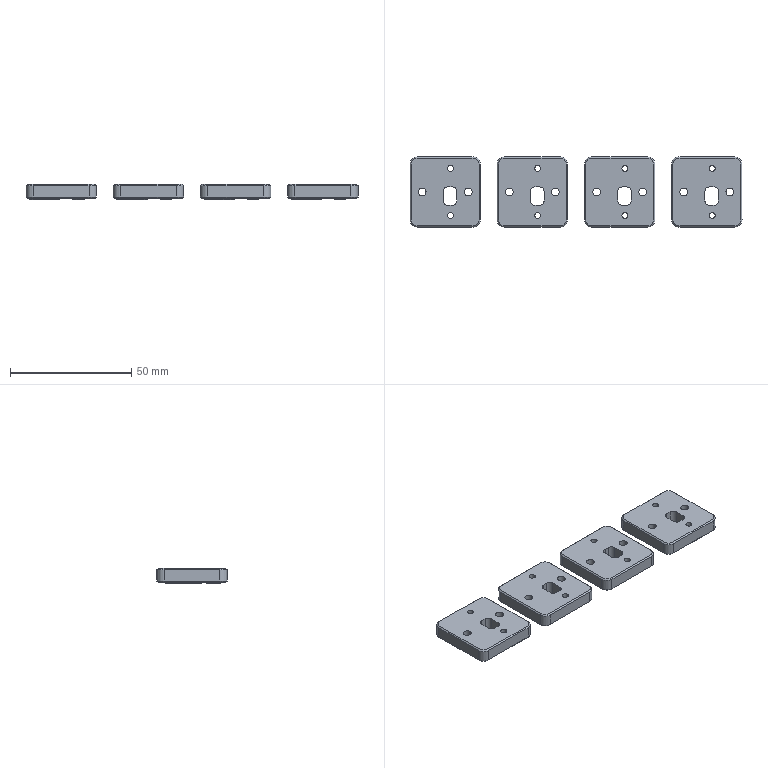NC program | NX | posted with a generic post | part box 137 x 29 x 6.3 mm
Lines 1 to 42 of 3650:
N10 G17 G21 G94 G90
(FLOOR_WALL_COPY , TOOL : D63)
N12 T01 M6
N14 G54
N16 G17 G0 G90 X103. Y0. S6500 M3
N18 G43 Z30. H1
N20 Z6.
N22 G94 G1 Z3. F1250.
N24 X100.
N26 X-100.
N28 X-103.
N30 Z6.
N32 G0 Z30.
N34 X103.
N36 Z5.
N38 G1 Z2.
N40 X100.
N42 X-100.
N44 X-103.
N46 Z5.
N48 G0 Z30.
N50 X103.
N52 Z4.
N54 G1 Z1.
N56 X100.
N58 X-100.
N60 X-103.
N62 Z4.
N64 G0 Z30.
N66 X103.
N68 Z3.
N70 G1 Z0.
N72 X100.
N74 X-100.
N76 X-103.
N78 Z3.
N80 G0 Z30.
N82 M5